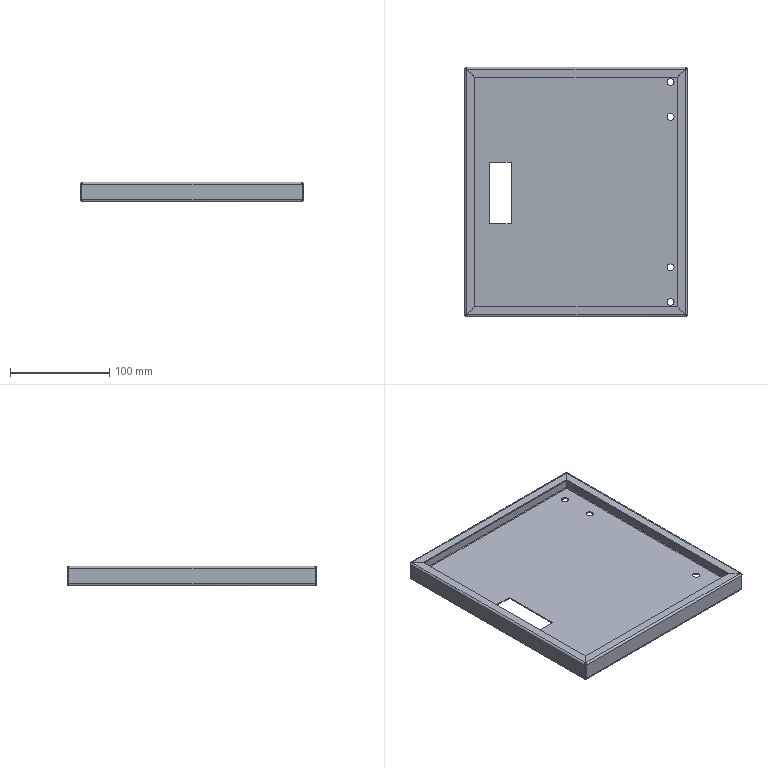Part | 1 solid | 82 faces | box 225 x 252 x 20 mm | volume 95766 mm3 | plane 42 | cylinder 24 | spline 16 | commonest cylinder face diameters 1.473 x8 3.873 x8 7 x8